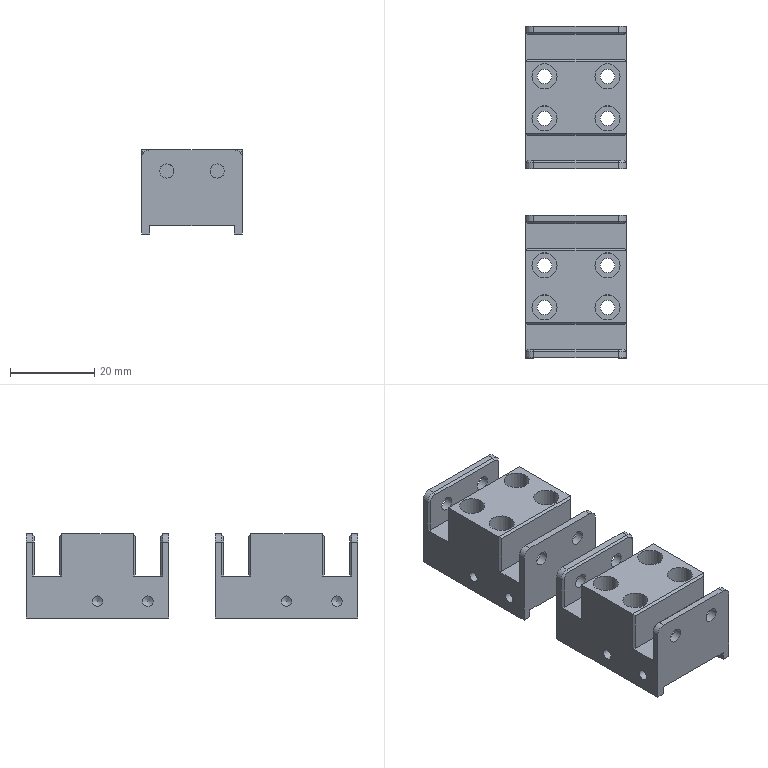Part | 2 solids | 124 faces | box 24 x 79 x 20 mm | volume 20350 mm3 | plane 68 | cylinder 40 | cone 16 | commonest cylinder face diameters 3.4 x16 2.5 x8 4 x8 6 x8